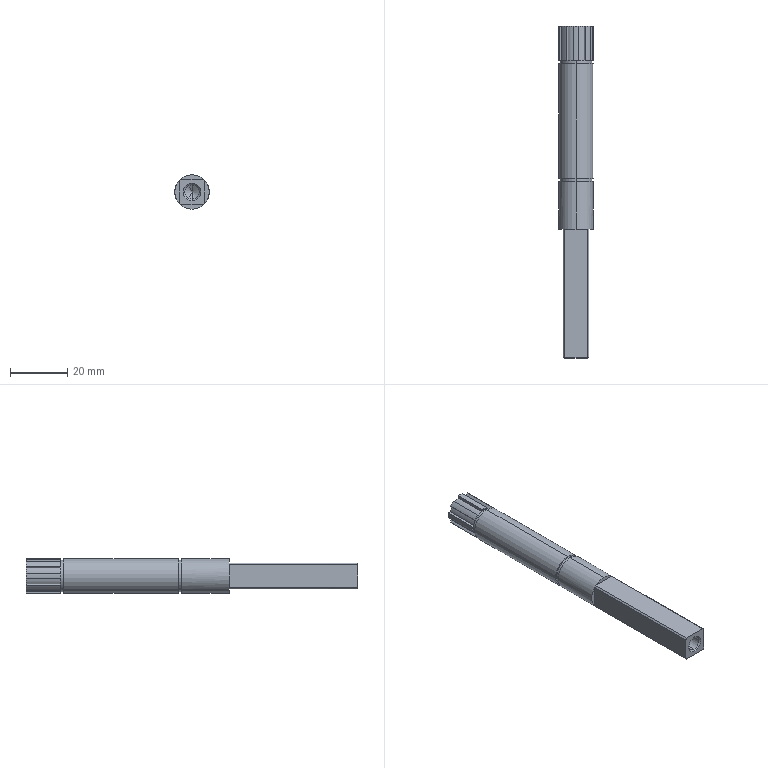Part | SolidWorks | features ICE 5, Extrusion 1, HoleWzd 1 | 1 solid | 76 faces | box 12 x 116 x 12 mm | volume 11161 mm3 | plane 46 | cylinder 26 | cone 4 | commonest cylinder face diameters 12 x12 10 x8 11 x4 5 x2